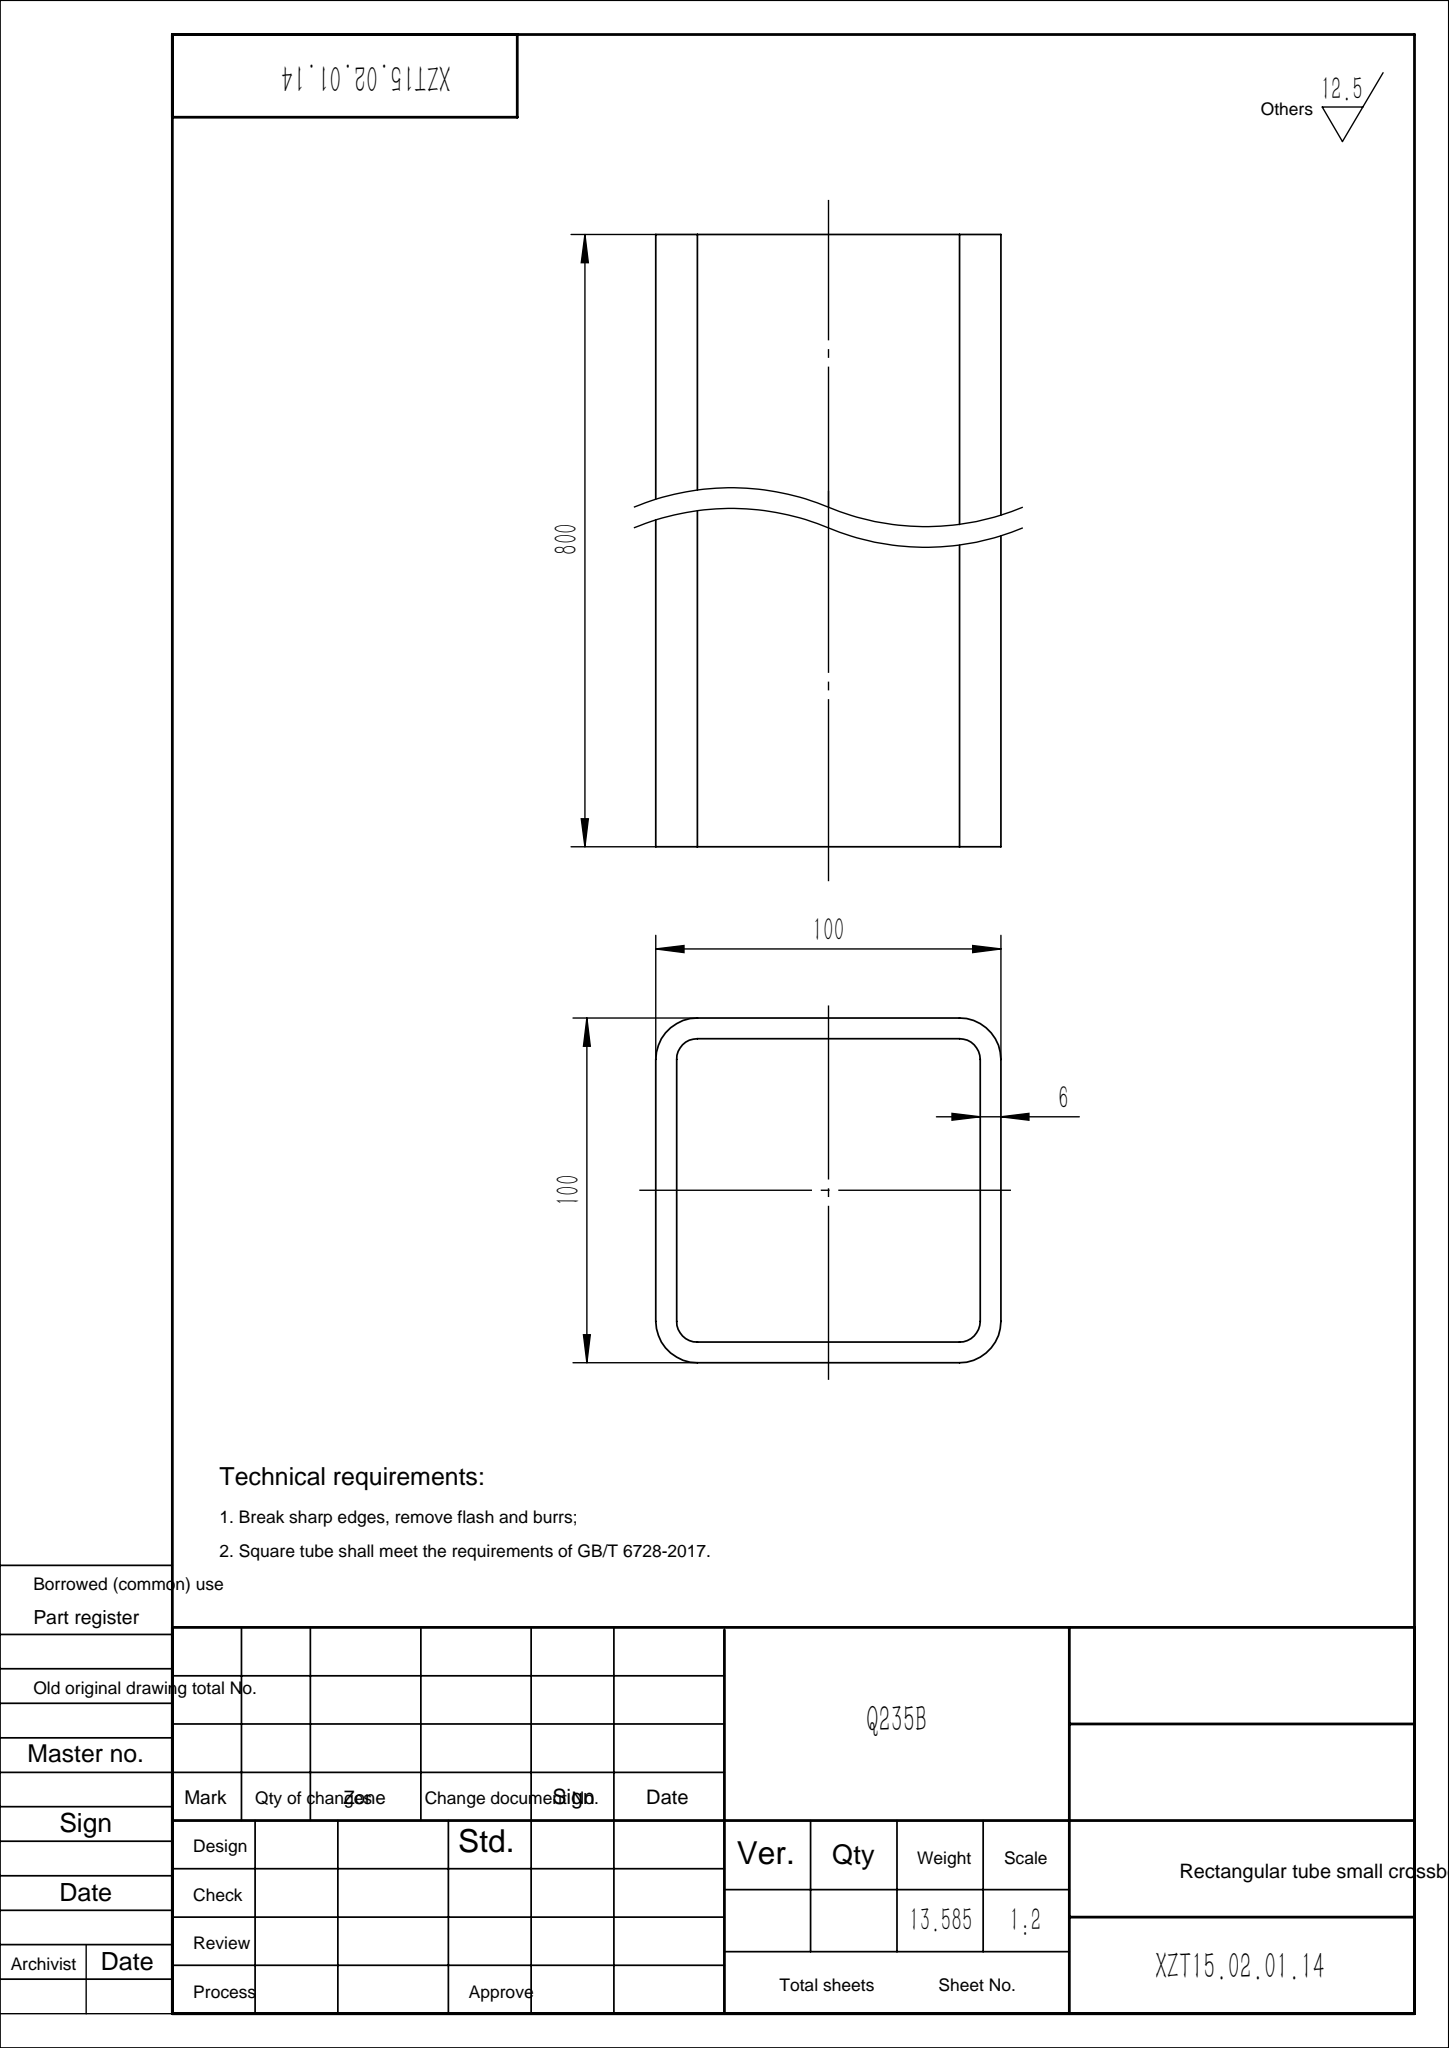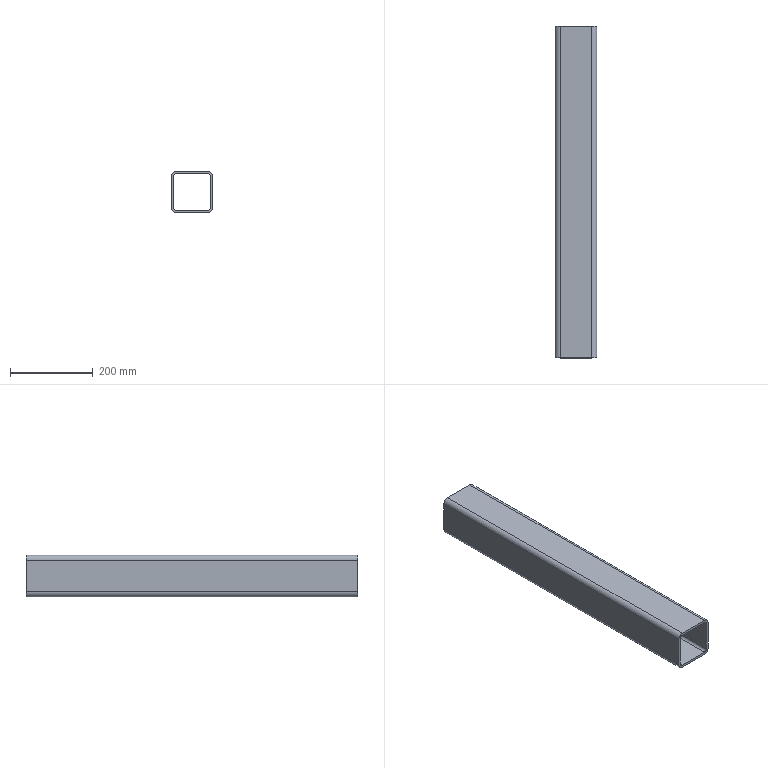Part | SolidWorks | features WeldMemberFeat 1, WeldmentFeature 1 | 1 solid | 18 faces | box 100 x 800 x 100 mm | volume 1730634 mm3 | plane 10 | cylinder 8 | commonest cylinder face diameters 12 x4 24 x4
STEP:
#1=CARTESIAN_POINT('',(-50.,0.,38.));
#2=VERTEX_POINT('',#1);
#3=CARTESIAN_POINT('',(-38.,0.,50.));
#4=VERTEX_POINT('',#3);
#5=CARTESIAN_POINT('',(-38.,0.,38.));
#6=DIRECTION('',(0.,1.,0.));
#7=DIRECTION('',(0.,0.,1.));
#8=AXIS2_PLACEMENT_3D('',#5,#6,#7);
#9=CIRCLE('',#8,12.);
#10=EDGE_CURVE('',#2,#4,#9,.T.);
#11=ORIENTED_EDGE('',*,*,#10,.T.);
#12=CARTESIAN_POINT('',(-38.,800.,50.));
#13=VERTEX_POINT('',#12);
#14=CARTESIAN_POINT('',(-38.,800.,50.));
#15=DIRECTION('',(0.,-1.,0.));
#16=VECTOR('',#15,1000.);
#17=LINE('',#14,#16);
#18=EDGE_CURVE('',#13,#4,#17,.T.);
#19=ORIENTED_EDGE('',*,*,#18,.F.);
#20=CARTESIAN_POINT('',(-50.,800.,38.));
#21=VERTEX_POINT('',#20);
#22=CARTESIAN_POINT('',(-38.,800.,38.));
#23=DIRECTION('',(0.,1.,0.));
#24=DIRECTION('',(0.,0.,1.));
#25=AXIS2_PLACEMENT_3D('',#22,#23,#24);
#26=CIRCLE('',#25,12.);
#27=EDGE_CURVE('',#21,#13,#26,.T.);
#28=ORIENTED_EDGE('',*,*,#27,.F.);
#29=CARTESIAN_POINT('',(-50.,800.,38.));
#30=DIRECTION('',(0.,-1.,0.));
#31=VECTOR('',#30,1000.);
#32=LINE('',#29,#31);
#33=EDGE_CURVE('',#21,#2,#32,.T.);
#34=ORIENTED_EDGE('',*,*,#33,.T.);
#35=EDGE_LOOP('',(#11,#19,#28,#34));
#36=FACE_OUTER_BOUND('',#35,.T.);
#37=CARTESIAN_POINT('',(-38.,800.,38.));
#38=DIRECTION('',(0.,-1.,0.));
#39=DIRECTION('',(0.,0.,-1.));
#40=AXIS2_PLACEMENT_3D('',#37,#38,#39);
#41=CYLINDRICAL_SURFACE('',#40,12.);
#42=ADVANCED_FACE('',(#36),#41,.T.);
#43=CARTESIAN_POINT('',(38.,0.,50.));
#44=VERTEX_POINT('',#43);
#45=CARTESIAN_POINT('',(-38.,0.,50.));
#46=DIRECTION('',(1.,0.,0.));
#47=VECTOR('',#46,1000.);
#48=LINE('',#45,#47);
#49=EDGE_CURVE('',#4,#44,#48,.T.);
#50=ORIENTED_EDGE('',*,*,#49,.T.);
#51=CARTESIAN_POINT('',(38.,800.,50.));
#52=VERTEX_POINT('',#51);
#53=CARTESIAN_POINT('',(38.,800.,50.));
#54=DIRECTION('',(0.,-1.,0.));
#55=VECTOR('',#54,1000.);
#56=LINE('',#53,#55);
#57=EDGE_CURVE('',#52,#44,#56,.T.);
#58=ORIENTED_EDGE('',*,*,#57,.F.);
#59=CARTESIAN_POINT('',(-38.,800.,50.));
#60=DIRECTION('',(1.,0.,0.));
#61=VECTOR('',#60,1000.);
#62=LINE('',#59,#61);
#63=EDGE_CURVE('',#13,#52,#62,.T.);
#64=ORIENTED_EDGE('',*,*,#63,.F.);
#65=ORIENTED_EDGE('',*,*,#18,.T.);
#66=EDGE_LOOP('',(#50,#58,#64,#65));
#67=FACE_OUTER_BOUND('',#66,.T.);
#68=CARTESIAN_POINT('',(-38.,800.,50.));
#69=DIRECTION('',(0.,0.,-1.));
#70=DIRECTION('',(-1.,0.,0.));
#71=AXIS2_PLACEMENT_3D('',#68,#69,#70);
#72=PLANE('',#71);
#73=ADVANCED_FACE('',(#67),#72,.F.);
#74=CARTESIAN_POINT('',(50.,0.,38.));
#75=VERTEX_POINT('',#74);
#76=CARTESIAN_POINT('',(38.,0.,38.));
#77=DIRECTION('',(0.,1.,0.));
#78=DIRECTION('',(0.,0.,1.));
#79=AXIS2_PLACEMENT_3D('',#76,#77,#78);
#80=CIRCLE('',#79,12.);
#81=EDGE_CURVE('',#44,#75,#80,.T.);
#82=ORIENTED_EDGE('',*,*,#81,.T.);
#83=CARTESIAN_POINT('',(50.,800.,38.));
#84=VERTEX_POINT('',#83);
#85=CARTESIAN_POINT('',(50.,800.,38.));
#86=DIRECTION('',(0.,-1.,0.));
#87=VECTOR('',#86,1000.);
#88=LINE('',#85,#87);
#89=EDGE_CURVE('',#84,#75,#88,.T.);
#90=ORIENTED_EDGE('',*,*,#89,.F.);
#91=CARTESIAN_POINT('',(38.,800.,38.));
#92=DIRECTION('',(0.,1.,0.));
#93=DIRECTION('',(0.,0.,1.));
#94=AXIS2_PLACEMENT_3D('',#91,#92,#93);
#95=CIRCLE('',#94,12.);
#96=EDGE_CURVE('',#52,#84,#95,.T.);
#97=ORIENTED_EDGE('',*,*,#96,.F.);
#98=ORIENTED_EDGE('',*,*,#57,.T.);
#99=EDGE_LOOP('',(#82,#90,#97,#98));
#100=FACE_OUTER_BOUND('',#99,.T.);
#101=CARTESIAN_POINT('',(38.,800.,38.));
#102=DIRECTION('',(0.,-1.,0.));
#103=DIRECTION('',(0.,0.,-1.));
#104=AXIS2_PLACEMENT_3D('',#101,#102,#103);
#105=CYLINDRICAL_SURFACE('',#104,12.);
#106=ADVANCED_FACE('',(#100),#105,.T.);
#107=CARTESIAN_POINT('',(50.,0.,-38.));
#108=VERTEX_POINT('',#107);
#109=CARTESIAN_POINT('',(50.,0.,-38.));
#110=DIRECTION('',(0.,0.,-1.));
#111=VECTOR('',#110,1000.);
#112=LINE('',#109,#111);
#113=EDGE_CURVE('',#75,#108,#112,.T.);
#114=ORIENTED_EDGE('',*,*,#113,.T.);
#115=CARTESIAN_POINT('',(50.,800.,-38.));
#116=VERTEX_POINT('',#115);
#117=CARTESIAN_POINT('',(50.,800.,-38.));
#118=DIRECTION('',(0.,-1.,0.));
#119=VECTOR('',#118,1000.);
#120=LINE('',#117,#119);
#121=EDGE_CURVE('',#116,#108,#120,.T.);
#122=ORIENTED_EDGE('',*,*,#121,.F.);
#123=CARTESIAN_POINT('',(50.,800.,-38.));
#124=DIRECTION('',(0.,0.,-1.));
#125=VECTOR('',#124,1000.);
#126=LINE('',#123,#125);
#127=EDGE_CURVE('',#84,#116,#126,.T.);
#128=ORIENTED_EDGE('',*,*,#127,.F.);
#129=ORIENTED_EDGE('',*,*,#89,.T.);
#130=EDGE_LOOP('',(#114,#122,#128,#129));
#131=FACE_OUTER_BOUND('',#130,.T.);
#132=CARTESIAN_POINT('',(50.,800.,-38.));
#133=DIRECTION('',(-1.,0.,0.));
#134=DIRECTION('',(0.,0.,1.));
#135=AXIS2_PLACEMENT_3D('',#132,#133,#134);
#136=PLANE('',#135);
#137=ADVANCED_FACE('',(#131),#136,.F.);
#138=CARTESIAN_POINT('',(38.,0.,-50.));
#139=VERTEX_POINT('',#138);
#140=CARTESIAN_POINT('',(38.,0.,-38.));
#141=DIRECTION('',(0.,1.,0.));
#142=DIRECTION('',(0.,0.,1.));
#143=AXIS2_PLACEMENT_3D('',#140,#141,#142);
#144=CIRCLE('',#143,12.);
#145=EDGE_CURVE('',#108,#139,#144,.T.);
#146=ORIENTED_EDGE('',*,*,#145,.T.);
#147=CARTESIAN_POINT('',(38.,800.,-50.));
#148=VERTEX_POINT('',#147);
#149=CARTESIAN_POINT('',(38.,800.,-50.));
#150=DIRECTION('',(0.,-1.,0.));
#151=VECTOR('',#150,1000.);
#152=LINE('',#149,#151);
#153=EDGE_CURVE('',#148,#139,#152,.T.);
#154=ORIENTED_EDGE('',*,*,#153,.F.);
#155=CARTESIAN_POINT('',(38.,800.,-38.));
#156=DIRECTION('',(0.,1.,0.));
#157=DIRECTION('',(0.,0.,1.));
#158=AXIS2_PLACEMENT_3D('',#155,#156,#157);
#159=CIRCLE('',#158,12.);
#160=EDGE_CURVE('',#116,#148,#159,.T.);
#161=ORIENTED_EDGE('',*,*,#160,.F.);
#162=ORIENTED_EDGE('',*,*,#121,.T.);
#163=EDGE_LOOP('',(#146,#154,#161,#162));
#164=FACE_OUTER_BOUND('',#163,.T.);
#165=CARTESIAN_POINT('',(38.,800.,-38.));
#166=DIRECTION('',(0.,-1.,0.));
#167=DIRECTION('',(0.,0.,-1.));
#168=AXIS2_PLACEMENT_3D('',#165,#166,#167);
#169=CYLINDRICAL_SURFACE('',#168,12.);
#170=ADVANCED_FACE('',(#164),#169,.T.);
#171=CARTESIAN_POINT('',(-38.,0.,-50.));
#172=VERTEX_POINT('',#171);
#173=CARTESIAN_POINT('',(38.,0.,-50.));
#174=DIRECTION('',(-1.,0.,0.));
#175=VECTOR('',#174,1000.);
#176=LINE('',#173,#175);
#177=EDGE_CURVE('',#139,#172,#176,.T.);
#178=ORIENTED_EDGE('',*,*,#177,.T.);
#179=CARTESIAN_POINT('',(-38.,800.,-50.));
#180=VERTEX_POINT('',#179);
#181=CARTESIAN_POINT('',(-38.,800.,-50.));
#182=DIRECTION('',(0.,-1.,0.));
#183=VECTOR('',#182,1000.);
#184=LINE('',#181,#183);
#185=EDGE_CURVE('',#180,#172,#184,.T.);
#186=ORIENTED_EDGE('',*,*,#185,.F.);
#187=CARTESIAN_POINT('',(38.,800.,-50.));
#188=DIRECTION('',(-1.,0.,0.));
#189=VECTOR('',#188,1000.);
#190=LINE('',#187,#189);
#191=EDGE_CURVE('',#148,#180,#190,.T.);
#192=ORIENTED_EDGE('',*,*,#191,.F.);
#193=ORIENTED_EDGE('',*,*,#153,.T.);
#194=EDGE_LOOP('',(#178,#186,#192,#193));
#195=FACE_OUTER_BOUND('',#194,.T.);
#196=CARTESIAN_POINT('',(38.,800.,-50.));
#197=DIRECTION('',(0.,0.,1.));
#198=DIRECTION('',(1.,0.,0.));
#199=AXIS2_PLACEMENT_3D('',#196,#197,#198);
#200=PLANE('',#199);
#201=ADVANCED_FACE('',(#195),#200,.F.);
#202=CARTESIAN_POINT('',(-50.,0.,-38.));
#203=VERTEX_POINT('',#202);
#204=CARTESIAN_POINT('',(-38.,0.,-38.));
#205=DIRECTION('',(0.,1.,0.));
#206=DIRECTION('',(0.,0.,1.));
#207=AXIS2_PLACEMENT_3D('',#204,#205,#206);
#208=CIRCLE('',#207,12.);
#209=EDGE_CURVE('',#172,#203,#208,.T.);
#210=ORIENTED_EDGE('',*,*,#209,.T.);
#211=CARTESIAN_POINT('',(-50.,800.,-38.));
#212=VERTEX_POINT('',#211);
#213=CARTESIAN_POINT('',(-50.,800.,-38.));
#214=DIRECTION('',(0.,-1.,0.));
#215=VECTOR('',#214,1000.);
#216=LINE('',#213,#215);
#217=EDGE_CURVE('',#212,#203,#216,.T.);
#218=ORIENTED_EDGE('',*,*,#217,.F.);
#219=CARTESIAN_POINT('',(-38.,800.,-38.));
#220=DIRECTION('',(0.,1.,0.));
#221=DIRECTION('',(0.,0.,1.));
#222=AXIS2_PLACEMENT_3D('',#219,#220,#221);
#223=CIRCLE('',#222,12.);
#224=EDGE_CURVE('',#180,#212,#223,.T.);
#225=ORIENTED_EDGE('',*,*,#224,.F.);
#226=ORIENTED_EDGE('',*,*,#185,.T.);
#227=EDGE_LOOP('',(#210,#218,#225,#226));
#228=FACE_OUTER_BOUND('',#227,.T.);
#229=CARTESIAN_POINT('',(-38.,800.,-38.));
#230=DIRECTION('',(0.,-1.,0.));
#231=DIRECTION('',(0.,0.,-1.));
#232=AXIS2_PLACEMENT_3D('',#229,#230,#231);
#233=CYLINDRICAL_SURFACE('',#232,12.);
#234=ADVANCED_FACE('',(#228),#233,.T.);
#235=CARTESIAN_POINT('',(38.,0.,44.));
#236=VERTEX_POINT('',#235);
#237=CARTESIAN_POINT('',(44.,0.,38.));
#238=VERTEX_POINT('',#237);
#239=CARTESIAN_POINT('',(38.,0.,38.));
#240=DIRECTION('',(0.,1.,0.));
#241=DIRECTION('',(0.,0.,1.));
#242=AXIS2_PLACEMENT_3D('',#239,#240,#241);
#243=CIRCLE('',#242,6.);
#244=EDGE_CURVE('',#236,#238,#243,.T.);
#245=ORIENTED_EDGE('',*,*,#244,.F.);
#246=CARTESIAN_POINT('',(38.,800.,44.));
#247=VERTEX_POINT('',#246);
#248=CARTESIAN_POINT('',(38.,800.,44.));
#249=DIRECTION('',(0.,-1.,0.));
#250=VECTOR('',#249,1000.);
#251=LINE('',#248,#250);
#252=EDGE_CURVE('',#247,#236,#251,.T.);
#253=ORIENTED_EDGE('',*,*,#252,.F.);
#254=CARTESIAN_POINT('',(44.,800.,38.));
#255=VERTEX_POINT('',#254);
#256=CARTESIAN_POINT('',(38.,800.,38.));
#257=DIRECTION('',(0.,1.,0.));
#258=DIRECTION('',(0.,0.,1.));
#259=AXIS2_PLACEMENT_3D('',#256,#257,#258);
#260=CIRCLE('',#259,6.);
#261=EDGE_CURVE('',#247,#255,#260,.T.);
#262=ORIENTED_EDGE('',*,*,#261,.T.);
#263=CARTESIAN_POINT('',(44.,800.,38.));
#264=DIRECTION('',(0.,-1.,0.));
#265=VECTOR('',#264,1000.);
#266=LINE('',#263,#265);
#267=EDGE_CURVE('',#255,#238,#266,.T.);
#268=ORIENTED_EDGE('',*,*,#267,.T.);
#269=EDGE_LOOP('',(#245,#253,#262,#268));
#270=FACE_OUTER_BOUND('',#269,.T.);
#271=CARTESIAN_POINT('',(38.,800.,38.));
#272=DIRECTION('',(0.,-1.,0.));
#273=DIRECTION('',(0.,0.,-1.));
#274=AXIS2_PLACEMENT_3D('',#271,#272,#273);
#275=CYLINDRICAL_SURFACE('',#274,6.);
#276=ADVANCED_FACE('',(#270),#275,.F.);
#277=CARTESIAN_POINT('',(-38.,0.,44.));
#278=VERTEX_POINT('',#277);
#279=CARTESIAN_POINT('',(-38.,0.,44.));
#280=DIRECTION('',(1.,0.,0.));
#281=VECTOR('',#280,1000.);
#282=LINE('',#279,#281);
#283=EDGE_CURVE('',#278,#236,#282,.T.);
#284=ORIENTED_EDGE('',*,*,#283,.F.);
#285=CARTESIAN_POINT('',(-38.,800.,44.));
#286=VERTEX_POINT('',#285);
#287=CARTESIAN_POINT('',(-38.,800.,44.));
#288=DIRECTION('',(0.,-1.,0.));
#289=VECTOR('',#288,1000.);
#290=LINE('',#287,#289);
#291=EDGE_CURVE('',#286,#278,#290,.T.);
#292=ORIENTED_EDGE('',*,*,#291,.F.);
#293=CARTESIAN_POINT('',(-38.,800.,44.));
#294=DIRECTION('',(1.,0.,0.));
#295=VECTOR('',#294,1000.);
#296=LINE('',#293,#295);
#297=EDGE_CURVE('',#286,#247,#296,.T.);
#298=ORIENTED_EDGE('',*,*,#297,.T.);
#299=ORIENTED_EDGE('',*,*,#252,.T.);
#300=EDGE_LOOP('',(#284,#292,#298,#299));
#301=FACE_OUTER_BOUND('',#300,.T.);
#302=CARTESIAN_POINT('',(-38.,800.,44.));
#303=DIRECTION('',(0.,0.,-1.));
#304=DIRECTION('',(-1.,0.,0.));
#305=AXIS2_PLACEMENT_3D('',#302,#303,#304);
#306=PLANE('',#305);
#307=ADVANCED_FACE('',(#301),#306,.T.);
#308=CARTESIAN_POINT('',(-44.,0.,38.));
#309=VERTEX_POINT('',#308);
#310=CARTESIAN_POINT('',(-38.,0.,38.));
#311=DIRECTION('',(0.,1.,0.));
#312=DIRECTION('',(0.,0.,1.));
#313=AXIS2_PLACEMENT_3D('',#310,#311,#312);
#314=CIRCLE('',#313,6.);
#315=EDGE_CURVE('',#309,#278,#314,.T.);
#316=ORIENTED_EDGE('',*,*,#315,.F.);
#317=CARTESIAN_POINT('',(-44.,800.,38.));
#318=VERTEX_POINT('',#317);
#319=CARTESIAN_POINT('',(-44.,800.,38.));
#320=DIRECTION('',(0.,-1.,0.));
#321=VECTOR('',#320,1000.);
#322=LINE('',#319,#321);
#323=EDGE_CURVE('',#318,#309,#322,.T.);
#324=ORIENTED_EDGE('',*,*,#323,.F.);
#325=CARTESIAN_POINT('',(-38.,800.,38.));
#326=DIRECTION('',(0.,1.,0.));
#327=DIRECTION('',(0.,0.,1.));
#328=AXIS2_PLACEMENT_3D('',#325,#326,#327);
#329=CIRCLE('',#328,6.);
#330=EDGE_CURVE('',#318,#286,#329,.T.);
#331=ORIENTED_EDGE('',*,*,#330,.T.);
#332=ORIENTED_EDGE('',*,*,#291,.T.);
#333=EDGE_LOOP('',(#316,#324,#331,#332));
#334=FACE_OUTER_BOUND('',#333,.T.);
#335=CARTESIAN_POINT('',(-38.,800.,38.));
#336=DIRECTION('',(0.,-1.,0.));
#337=DIRECTION('',(0.,0.,-1.));
#338=AXIS2_PLACEMENT_3D('',#335,#336,#337);
#339=CYLINDRICAL_SURFACE('',#338,6.);
#340=ADVANCED_FACE('',(#334),#339,.F.);
#341=CARTESIAN_POINT('',(-44.,0.,-38.));
#342=VERTEX_POINT('',#341);
#343=CARTESIAN_POINT('',(-44.,0.,38.));
#344=DIRECTION('',(0.,0.,1.));
#345=VECTOR('',#344,1000.);
#346=LINE('',#343,#345);
#347=EDGE_CURVE('',#342,#309,#346,.T.);
#348=ORIENTED_EDGE('',*,*,#347,.F.);
#349=CARTESIAN_POINT('',(-44.,800.,-38.));
#350=VERTEX_POINT('',#349);
#351=CARTESIAN_POINT('',(-44.,800.,-38.));
#352=DIRECTION('',(0.,-1.,0.));
#353=VECTOR('',#352,1000.);
#354=LINE('',#351,#353);
#355=EDGE_CURVE('',#350,#342,#354,.T.);
#356=ORIENTED_EDGE('',*,*,#355,.F.);
#357=CARTESIAN_POINT('',(-44.,800.,38.));
#358=DIRECTION('',(0.,0.,1.));
#359=VECTOR('',#358,1000.);
#360=LINE('',#357,#359);
#361=EDGE_CURVE('',#350,#318,#360,.T.);
#362=ORIENTED_EDGE('',*,*,#361,.T.);
#363=ORIENTED_EDGE('',*,*,#323,.T.);
#364=EDGE_LOOP('',(#348,#356,#362,#363));
#365=FACE_OUTER_BOUND('',#364,.T.);
#366=CARTESIAN_POINT('',(-44.,800.,38.));
#367=DIRECTION('',(1.,0.,0.));
#368=DIRECTION('',(0.,0.,-1.));
#369=AXIS2_PLACEMENT_3D('',#366,#367,#368);
#370=PLANE('',#369);
#371=ADVANCED_FACE('',(#365),#370,.T.);
#372=CARTESIAN_POINT('',(-38.,0.,-44.));
#373=VERTEX_POINT('',#372);
#374=CARTESIAN_POINT('',(-38.,0.,-38.));
#375=DIRECTION('',(0.,1.,0.));
#376=DIRECTION('',(0.,0.,1.));
#377=AXIS2_PLACEMENT_3D('',#374,#375,#376);
#378=CIRCLE('',#377,6.);
#379=EDGE_CURVE('',#373,#342,#378,.T.);
#380=ORIENTED_EDGE('',*,*,#379,.F.);
#381=CARTESIAN_POINT('',(-38.,800.,-44.));
#382=VERTEX_POINT('',#381);
#383=CARTESIAN_POINT('',(-38.,800.,-44.));
#384=DIRECTION('',(0.,-1.,0.));
#385=VECTOR('',#384,1000.);
#386=LINE('',#383,#385);
#387=EDGE_CURVE('',#382,#373,#386,.T.);
#388=ORIENTED_EDGE('',*,*,#387,.F.);
#389=CARTESIAN_POINT('',(-38.,800.,-38.));
#390=DIRECTION('',(0.,1.,0.));
#391=DIRECTION('',(0.,0.,1.));
#392=AXIS2_PLACEMENT_3D('',#389,#390,#391);
#393=CIRCLE('',#392,6.);
#394=EDGE_CURVE('',#382,#350,#393,.T.);
#395=ORIENTED_EDGE('',*,*,#394,.T.);
#396=ORIENTED_EDGE('',*,*,#355,.T.);
#397=EDGE_LOOP('',(#380,#388,#395,#396));
#398=FACE_OUTER_BOUND('',#397,.T.);
#399=CARTESIAN_POINT('',(-38.,800.,-38.));
#400=DIRECTION('',(0.,-1.,0.));
#401=DIRECTION('',(0.,0.,-1.));
#402=AXIS2_PLACEMENT_3D('',#399,#400,#401);
#403=CYLINDRICAL_SURFACE('',#402,6.);
#404=ADVANCED_FACE('',(#398),#403,.F.);
#405=CARTESIAN_POINT('',(38.,0.,-44.));
#406=VERTEX_POINT('',#405);
#407=CARTESIAN_POINT('',(38.,0.,-44.));
#408=DIRECTION('',(-1.,0.,0.));
#409=VECTOR('',#408,1000.);
#410=LINE('',#407,#409);
#411=EDGE_CURVE('',#406,#373,#410,.T.);
#412=ORIENTED_EDGE('',*,*,#411,.F.);
#413=CARTESIAN_POINT('',(38.,800.,-44.));
#414=VERTEX_POINT('',#413);
#415=CARTESIAN_POINT('',(38.,800.,-44.));
#416=DIRECTION('',(0.,-1.,0.));
#417=VECTOR('',#416,1000.);
#418=LINE('',#415,#417);
#419=EDGE_CURVE('',#414,#406,#418,.T.);
#420=ORIENTED_EDGE('',*,*,#419,.F.);
#421=CARTESIAN_POINT('',(38.,800.,-44.));
#422=DIRECTION('',(-1.,0.,0.));
#423=VECTOR('',#422,1000.);
#424=LINE('',#421,#423);
#425=EDGE_CURVE('',#414,#382,#424,.T.);
#426=ORIENTED_EDGE('',*,*,#425,.T.);
#427=ORIENTED_EDGE('',*,*,#387,.T.);
#428=EDGE_LOOP('',(#412,#420,#426,#427));
#429=FACE_OUTER_BOUND('',#428,.T.);
#430=CARTESIAN_POINT('',(38.,800.,-44.));
#431=DIRECTION('',(0.,0.,1.));
#432=DIRECTION('',(1.,0.,0.));
#433=AXIS2_PLACEMENT_3D('',#430,#431,#432);
#434=PLANE('',#433);
#435=ADVANCED_FACE('',(#429),#434,.T.);
#436=CARTESIAN_POINT('',(44.,0.,-38.));
#437=VERTEX_POINT('',#436);
#438=CARTESIAN_POINT('',(38.,0.,-38.));
#439=DIRECTION('',(0.,1.,0.));
#440=DIRECTION('',(0.,0.,1.));
#441=AXIS2_PLACEMENT_3D('',#438,#439,#440);
#442=CIRCLE('',#441,6.);
#443=EDGE_CURVE('',#437,#406,#442,.T.);
#444=ORIENTED_EDGE('',*,*,#443,.F.);
#445=CARTESIAN_POINT('',(44.,800.,-38.));
#446=VERTEX_POINT('',#445);
#447=CARTESIAN_POINT('',(44.,800.,-38.));
#448=DIRECTION('',(0.,-1.,0.));
#449=VECTOR('',#448,1000.);
#450=LINE('',#447,#449);
#451=EDGE_CURVE('',#446,#437,#450,.T.);
#452=ORIENTED_EDGE('',*,*,#451,.F.);
#453=CARTESIAN_POINT('',(38.,800.,-38.));
#454=DIRECTION('',(0.,1.,0.));
#455=DIRECTION('',(0.,0.,1.));
#456=AXIS2_PLACEMENT_3D('',#453,#454,#455);
#457=CIRCLE('',#456,6.);
#458=EDGE_CURVE('',#446,#414,#457,.T.);
#459=ORIENTED_EDGE('',*,*,#458,.T.);
#460=ORIENTED_EDGE('',*,*,#419,.T.);
#461=EDGE_LOOP('',(#444,#452,#459,#460));
#462=FACE_OUTER_BOUND('',#461,.T.);
#463=CARTESIAN_POINT('',(38.,800.,-38.));
#464=DIRECTION('',(0.,-1.,0.));
#465=DIRECTION('',(0.,0.,-1.));
#466=AXIS2_PLACEMENT_3D('',#463,#464,#465);
#467=CYLINDRICAL_SURFACE('',#466,6.);
#468=ADVANCED_FACE('',(#462),#467,.F.);
#469=CARTESIAN_POINT('',(44.,0.,-38.));
#470=DIRECTION('',(0.,0.,-1.));
#471=VECTOR('',#470,1000.);
#472=LINE('',#469,#471);
#473=EDGE_CURVE('',#238,#437,#472,.T.);
#474=ORIENTED_EDGE('',*,*,#473,.F.);
#475=ORIENTED_EDGE('',*,*,#267,.F.);
#476=CARTESIAN_POINT('',(44.,800.,-38.));
#477=DIRECTION('',(0.,0.,-1.));
#478=VECTOR('',#477,1000.);
#479=LINE('',#476,#478);
#480=EDGE_CURVE('',#255,#446,#479,.T.);
#481=ORIENTED_EDGE('',*,*,#480,.T.);
#482=ORIENTED_EDGE('',*,*,#451,.T.);
#483=EDGE_LOOP('',(#474,#475,#481,#482));
#484=FACE_OUTER_BOUND('',#483,.T.);
#485=CARTESIAN_POINT('',(44.,800.,-38.));
#486=DIRECTION('',(-1.,0.,0.));
#487=DIRECTION('',(0.,0.,1.));
#488=AXIS2_PLACEMENT_3D('',#485,#486,#487);
#489=PLANE('',#488);
#490=ADVANCED_FACE('',(#484),#489,.T.);
#491=CARTESIAN_POINT('',(-50.,0.,38.));
#492=DIRECTION('',(0.,0.,1.));
#493=VECTOR('',#492,1000.);
#494=LINE('',#491,#493);
#495=EDGE_CURVE('',#203,#2,#494,.T.);
#496=ORIENTED_EDGE('',*,*,#495,.T.);
#497=ORIENTED_EDGE('',*,*,#33,.F.);
#498=CARTESIAN_POINT('',(-50.,800.,38.));
#499=DIRECTION('',(0.,0.,1.));
#500=VECTOR('',#499,1000.);
#501=LINE('',#498,#500);
#502=EDGE_CURVE('',#212,#21,#501,.T.);
#503=ORIENTED_EDGE('',*,*,#502,.F.);
#504=ORIENTED_EDGE('',*,*,#217,.T.);
#505=EDGE_LOOP('',(#496,#497,#503,#504));
#506=FACE_OUTER_BOUND('',#505,.T.);
#507=CARTESIAN_POINT('',(-50.,800.,38.));
#508=DIRECTION('',(1.,0.,0.));
#509=DIRECTION('',(0.,0.,-1.));
#510=AXIS2_PLACEMENT_3D('',#507,#508,#509);
#511=PLANE('',#510);
#512=ADVANCED_FACE('',(#506),#511,.F.);
#513=ORIENTED_EDGE('',*,*,#261,.F.);
#514=ORIENTED_EDGE('',*,*,#297,.F.);
#515=ORIENTED_EDGE('',*,*,#330,.F.);
#516=ORIENTED_EDGE('',*,*,#361,.F.);
#517=ORIENTED_EDGE('',*,*,#394,.F.);
#518=ORIENTED_EDGE('',*,*,#425,.F.);
#519=ORIENTED_EDGE('',*,*,#458,.F.);
#520=ORIENTED_EDGE('',*,*,#480,.F.);
#521=EDGE_LOOP('',(#513,#514,#515,#516,#517,#518,#519,#520));
#522=FACE_BOUND('',#521,.T.);
#523=ORIENTED_EDGE('',*,*,#27,.T.);
#524=ORIENTED_EDGE('',*,*,#63,.T.);
#525=ORIENTED_EDGE('',*,*,#96,.T.);
#526=ORIENTED_EDGE('',*,*,#127,.T.);
#527=ORIENTED_EDGE('',*,*,#160,.T.);
#528=ORIENTED_EDGE('',*,*,#191,.T.);
#529=ORIENTED_EDGE('',*,*,#224,.T.);
#530=ORIENTED_EDGE('',*,*,#502,.T.);
#531=EDGE_LOOP('',(#523,#524,#525,#526,#527,#528,#529,#530));
#532=FACE_OUTER_BOUND('',#531,.T.);
#533=CARTESIAN_POINT('',(-38.,800.,38.));
#534=DIRECTION('',(0.,1.,0.));
#535=DIRECTION('',(0.,0.,1.));
#536=AXIS2_PLACEMENT_3D('',#533,#534,#535);
#537=PLANE('',#536);
#538=ADVANCED_FACE('',(#522,#532),#537,.T.);
#539=ORIENTED_EDGE('',*,*,#244,.T.);
#540=ORIENTED_EDGE('',*,*,#473,.T.);
#541=ORIENTED_EDGE('',*,*,#443,.T.);
#542=ORIENTED_EDGE('',*,*,#411,.T.);
#543=ORIENTED_EDGE('',*,*,#379,.T.);
#544=ORIENTED_EDGE('',*,*,#347,.T.);
#545=ORIENTED_EDGE('',*,*,#315,.T.);
#546=ORIENTED_EDGE('',*,*,#283,.T.);
#547=EDGE_LOOP('',(#539,#540,#541,#542,#543,#544,#545,#546));
#548=FACE_BOUND('',#547,.T.);
#549=ORIENTED_EDGE('',*,*,#10,.F.);
#550=ORIENTED_EDGE('',*,*,#495,.F.);
#551=ORIENTED_EDGE('',*,*,#209,.F.);
#552=ORIENTED_EDGE('',*,*,#177,.F.);
#553=ORIENTED_EDGE('',*,*,#145,.F.);
#554=ORIENTED_EDGE('',*,*,#113,.F.);
#555=ORIENTED_EDGE('',*,*,#81,.F.);
#556=ORIENTED_EDGE('',*,*,#49,.F.);
#557=EDGE_LOOP('',(#549,#550,#551,#552,#553,#554,#555,#556));
#558=FACE_OUTER_BOUND('',#557,.T.);
#559=CARTESIAN_POINT('',(-38.,0.,38.));
#560=DIRECTION('',(0.,1.,0.));
#561=DIRECTION('',(0.,0.,1.));
#562=AXIS2_PLACEMENT_3D('',#559,#560,#561);
#563=PLANE('',#562);
#564=ADVANCED_FACE('',(#548,#558),#563,.F.);
#565=CLOSED_SHELL('',(#42,#73,#106,#137,#170,#201,#234,#276,#307,#340,#371,#404,#435,#468,#490,#512,#538,#564));
#566=MANIFOLD_SOLID_BREP('',#565);
#567=CARTESIAN_POINT('',(0.,0.,0.));
#568=DIRECTION('',(0.,0.,1.));
#569=DIRECTION('',(1.,0.,0.));
#570=AXIS2_PLACEMENT_3D('',#567,#568,#569);
#571=(LENGTH_UNIT()NAMED_UNIT(*)SI_UNIT(.MILLI.,.METRE.));
#572=UNCERTAINTY_MEASURE_WITH_UNIT(LENGTH_MEASURE(0.00001),#571,'','');
#573=(NAMED_UNIT(*)PLANE_ANGLE_UNIT()SI_UNIT($,.RADIAN.));
#574=(NAMED_UNIT(*)SI_UNIT($,.STERADIAN.)SOLID_ANGLE_UNIT());
#575=(GEOMETRIC_REPRESENTATION_CONTEXT(3)GLOBAL_UNCERTAINTY_ASSIGNED_CONTEXT((#572))GLOBAL_UNIT_ASSIGNED_CONTEXT((#571,#573,#574))REPRESENTATION_CONTEXT('',''));
#576=ADVANCED_BREP_SHAPE_REPRESENTATION('',(#566,#570),#575);